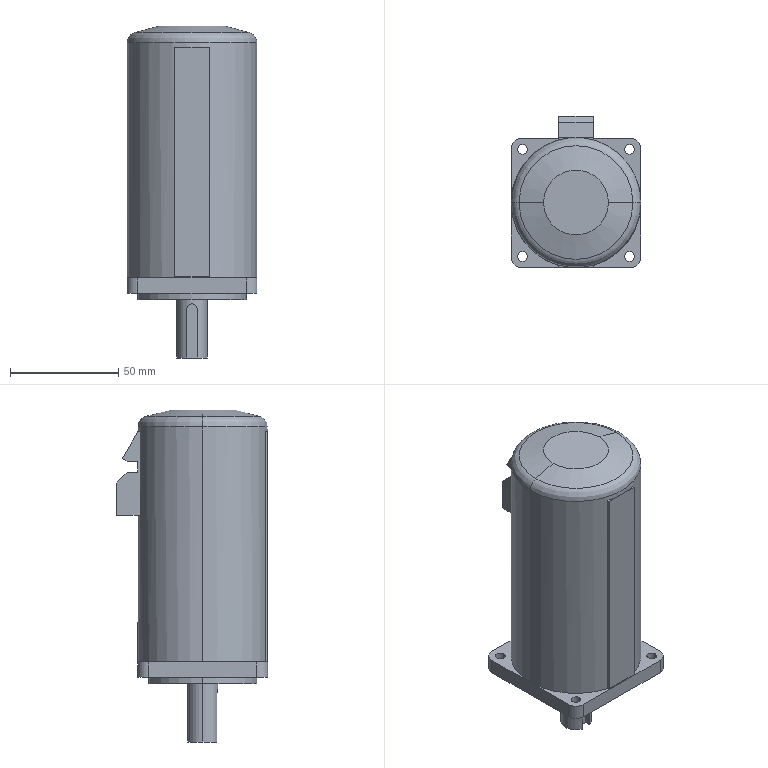Part | NX | 1 solid | 58 faces | box 60 x 70 x 153.5 mm | volume 363124 mm3 | plane 34 | cylinder 20 | torus 2 | cone 2 | commonest cylinder face diameters 4.5 x8 10 x4 60 x3 14 x2 50 x2 5 x1